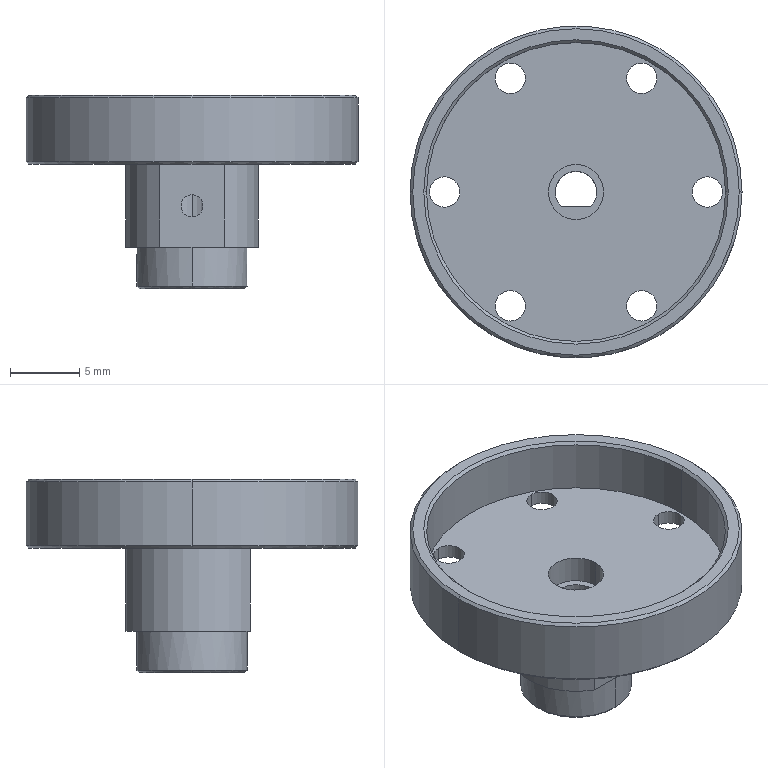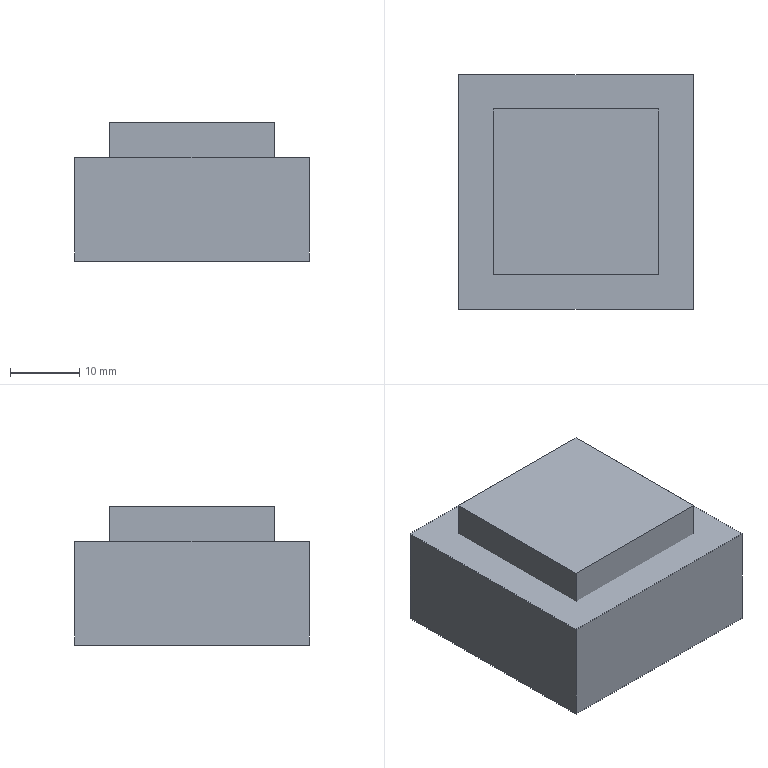CAM job | NX | 3-axis milling, drilling | part box 24 x 24 x 14 mm | stock box 34 x 34 x 20 mm
Tools:
number,name,description,diameter,corner_radius,flute_length,length,flutes
19,D80,Milling Tool-5 Parameters,80.0,0.0,50.0,75.0,2
15,D10,Milling Tool-5 Parameters,10.0,0.0,50.0,75.0,2
14,D10JING,Milling Tool-5 Parameters,10.0,0.0,50.0,75.0,2
1,D6A45,Milling Tool-5 Parameters,6.0,0.0,50.0,75.0,2
16,D3,Milling Tool-5 Parameters,3.0,0.0,50.0,75.0,2
17,1.25ZT,Drilling Tool,1.25,0.0,35.0,50.0,2
18,2.2ZT,Drilling Tool,2.2,0.0,35.0,50.0,2
24,D2,Milling Tool-5 Parameters,2.0,0.0,50.0,75.0,2
23,D1,Milling Tool-5 Parameters,1.0,0.0,50.0,75.0,2
Operations:
program,operation,operation_type,tool,method,geometry_group,spindle_rpm,surface_speed,feed_per_tooth,feed_cut,feed_plunge,cut_length_mm,path_length_mm,cut_time_min,machine_time_min
1,FLOOR_WALL,VolumeBased25DMillingOperation,D80,METHOD,A,6500.0,1633.0,0.1154,1500.0,100.0,126.0,180.0,0.084,0.0894
1,ADAPTIVE_MILLING,CavityMilling,D10,METHOD,A,9500.0,298.0,0.1579,3000.0,1000.0,916.804,998.804,0.3076,0.3158
1,ADAPTIVE_MILLING_COPY,CavityMilling,D10,METHOD,A,9500.0,298.0,0.1579,3000.0,1000.0,526.576,584.426,0.4372,0.443
1,ZLEVEL_PROFILE_COPY_1_COPY_COPY_1,ZLevelMilling,D10JING,METHOD,A,9500.0,298.0,0.0632,1200.0,1000.0,114.199,200.199,0.0958,0.1044
1,FLOOR_WALL_1,VolumeBased25DMillingOperation,D10JING,METHOD,A,9500.0,298.0,0.0658,1250.0,100.0,93.243,155.243,0.0746,0.0808
1,HOLE_MILLING,CylinderMilling,D3,METHOD,A,9500.0,89.0,0.0658,1250.0,100.0,44.062,113.562,0.0352,0.0422
1,PLANAR_MILL_COPY_COPY_COPY_COPY_COPY_COPY_1,PlanarMilling,D6A45,METHOD,A,9500.0,179.0,0.0658,1250.0,100.0,153.445,294.311,0.1228,0.1368
1,刀补,VolumeBased25DMillingOperation,D10JING,METHOD,A,9500.0,298.0,0.0658,1250.0,100.0,48.128,110.128,0.0385,0.0447
2,FLOOR_WALL_COPY,VolumeBased25DMillingOperation,D80,METHOD,B,6500.0,1633.0,0.1154,1500.0,100.0,696.0,1540.002,0.464,0.5484
2,FLOOR_WALL_2,VolumeBased25DMillingOperation,D10,METHOD,B,9500.0,298.0,0.1053,2000.0,1000.0,4637.005,4845.718,2.351,2.372
2,FLOOR_WALL_2_COPY,VolumeBased25DMillingOperation,D10,METHOD,B,9500.0,298.0,0.1053,2000.0,1000.0,386.216,460.643,0.2039,0.2113
2,FLOOR_WALL_1_COPY,VolumeBased25DMillingOperation,D10JING,METHOD,B,9500.0,298.0,0.0658,1250.0,100.0,141.886,213.886,0.1135,0.1207
2,DRILLING,Operation,D6A45,METHOD,B,5000.0,94.0,0.035,350.0,0.0,7.45,84.165,0.0213,0.029
2,DRILLING_COPY,Operation,D6A45,METHOD,B,5000.0,94.0,0.035,350.0,0.0,25.2,193.212,0.072,0.0888
2,DRILLING_COPY_1,Operation,1.25ZT,METHOD,B,2000.0,7.0,0.03,120.0,0.0,15.251,99.767,0.1271,0.1355
2,DRILLING_COPY_1_COPY,Operation,2.2ZT,METHOD,B,2000.0,7.0,0.03,120.0,0.0,36.966,243.797,0.308,0.3287
2,ZLEVEL_PROFILE,ZLevelMilling,D2,METHOD,B,9500.0,59.0,0.0526,1000.0,100.0,117.488,184.488,0.1175,0.1242
2,ZLEVEL_PROFILE_COPY,ZLevelMilling,D1,METHOD,B,9500.0,29.0,0.0421,800.0,100.0,329.824,630.03,0.4123,0.4423
2,PLANAR_MILL_COPY_COPY_COPY_COPY_COPY_COPY_1_COPY,PlanarMilling,D6A45,METHOD,B,9500.0,179.0,0.0658,1250.0,100.0,35.254,94.254,0.0282,0.0341
2,PLANAR_MILL_COPY_COPY_COPY_COPY_COPY_COPY_1_COPY_COPY,PlanarMilling,D6A45,METHOD,B,9500.0,179.0,0.0658,1250.0,100.0,85.519,162.519,0.0684,0.0761
2,刀补14,VolumeBased25DMillingOperation,D10JING,METHOD,B,9500.0,298.0,0.0658,1250.0,100.0,70.466,130.466,0.0564,0.0624
2,刀补24,ZLevelMilling,D2,METHOD,B,9500.0,59.0,0.0526,1000.0,100.0,16.44,84.44,0.0164,0.0232